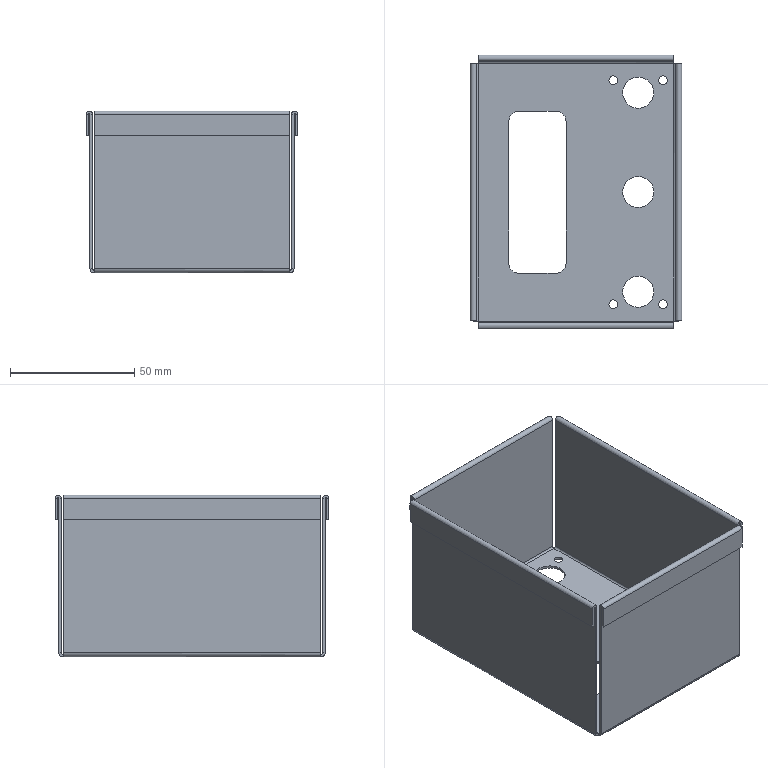Part | STEP file | X77-08307 | 1 solid | 92 faces | box 85 x 110 x 65 mm | volume 33590 mm3 | plane 50 | cylinder 34 | spline 8 | commonest cylinder face diameters 3.5 x8 12.5 x6 0.5 x4 1.473 x4 2.5 x4 3.473 x4